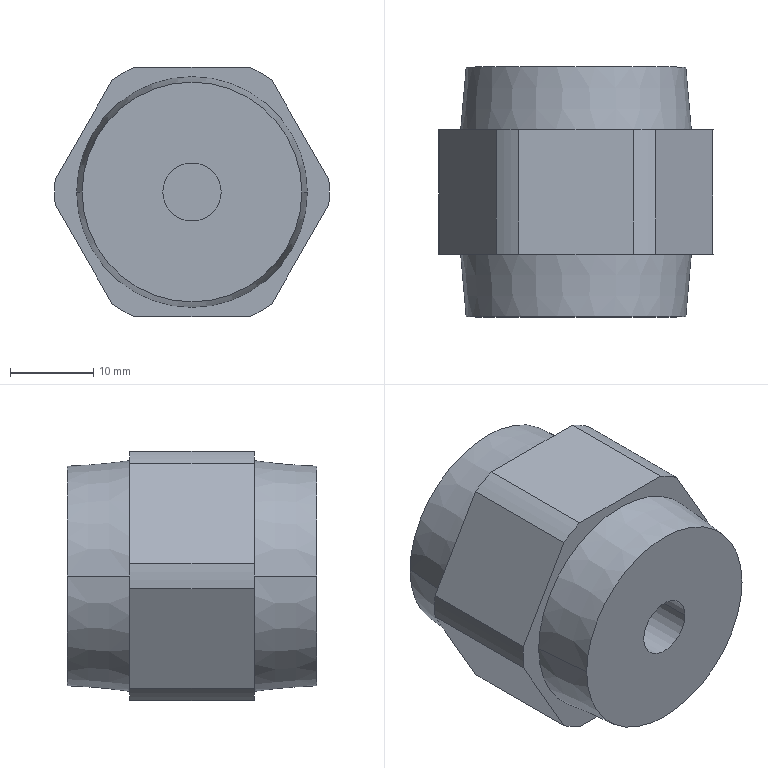Part | STEP file | SOLID | 1 solid | 26 faces | box 33 x 30 x 30 mm | volume 19613 mm3 | plane 12 | cylinder 10 | cone 4 | commonest cylinder face diameters 33 x6 7 x4